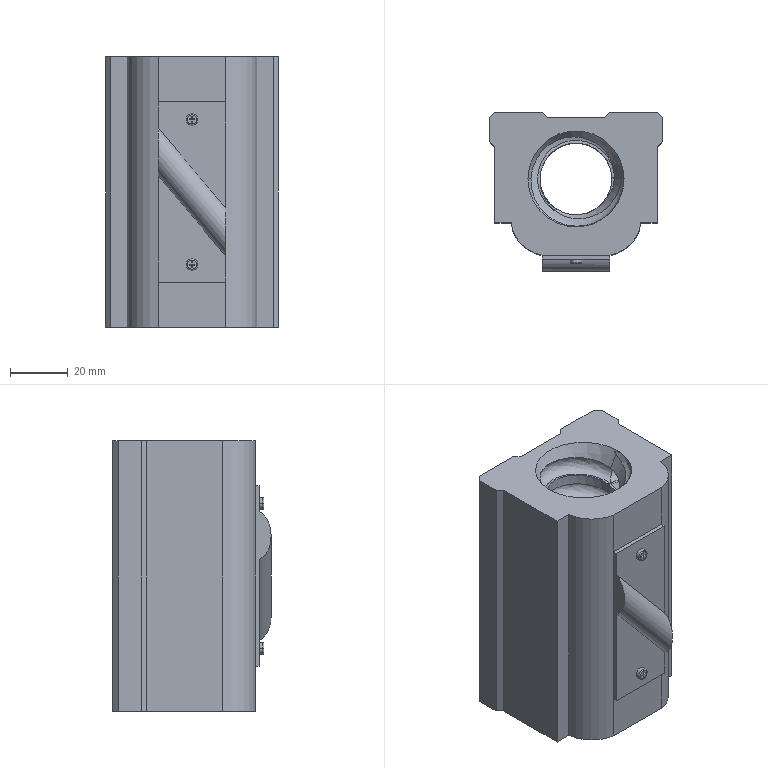Part | SolidWorks | features BaseBody 1 | 1 solid | 294 faces | box 60 x 55 x 94 mm | volume 177784 mm3 | cylinder 171 | spline 58 | plane 53 | cone 12 | commonest cylinder face diameters 6.647 x84 8 x80 4 x4 25.58 x2 11 x1